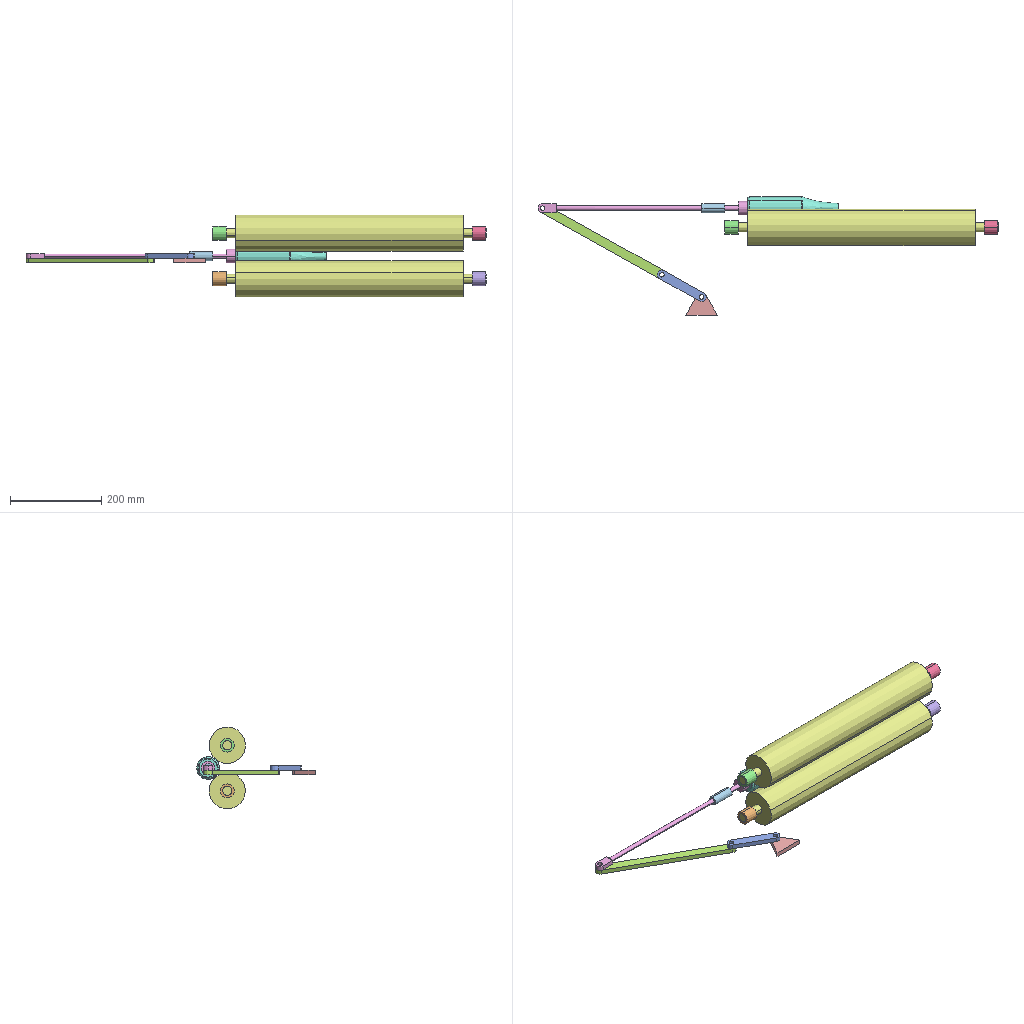Assembly | SolidWorks | 8 different items | 9 placed | box 1010 x 260 x 179 mm
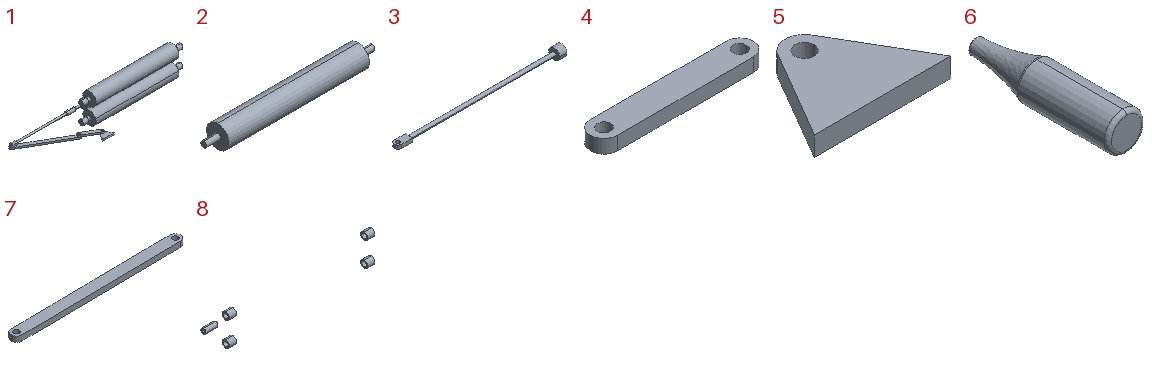Parts list (item | name | quantity | size | volume | features):
1 | (subassembly) | x1 | 990 x 265 x 180 mm | 5381178 mm3 | -
2 | - | x2 | 600 x 80 x 80 mm | 2544690 mm3 | features Revolution 1
3 | - | x1 | 460 x 30 x 30 mm | 52338 mm3 | features Extrusion 1, Revolution 1
4 | - | x1 | 120 x 20 x 10 mm | 21571 mm3 | features Extrusion 1
5 | - | x1 | 70 x 50 x 10 mm | 19476 mm3 | features Extrusion 1
6 | - | x1 | 50 x 200 x 50 mm | 77937 mm3 | features Fillet 2, Revolution 1, Shell 1
7 | - | x1 | 319.982 x 23.296 x 10 mm | 61571 mm3 | features Extrusion 1
8 | - | x1 | 650 x 67 x 130 mm | 58905 mm3 | features ICE 1, MirrorSolid 1, Revolution 1
Mates (type | each side: item.copy, entity, surface, feature):
Concentric | 5.1 face cylinder Boss-Extrude1 | 4.1 face cylinder Boss-Extrude1
Coincident | 5.1 face plane Boss-Extrude1 | 4.1 face plane Boss-Extrude1
Coincident | 4.1 face plane Boss-Extrude1 | 7.1 face plane Boss-Extrude1
Concentric | 4.1 face cylinder Boss-Extrude1 | 7.1 face cylinder Boss-Extrude1
Concentric | 7.1 face cylinder Boss-Extrude1 | 3.1 face cylinder Boss-Extrude1
Coincident | 7.1 face plane Boss-Extrude1 | 3.1 face plane Boss-Extrude1
Concentric | 8.1 face cylinder Mirror5 | 2.1 face cylinder Revolve1
Coincident | 8.1 face plane Mirror5 | 2.1 face plane Revolve1
Concentric | 8.1 face cylinder Revolve1 | 2.2 face cylinder Revolve1
Coincident | 8.1 face plane Revolve1 | 2.2 face plane Revolve1
Concentric | 3.1 face cylinder Revolve1 | 8.1 face cylinder Boss-Extrude1
Parallel | 8.1 plane | 5.1 face plane Boss-Extrude1